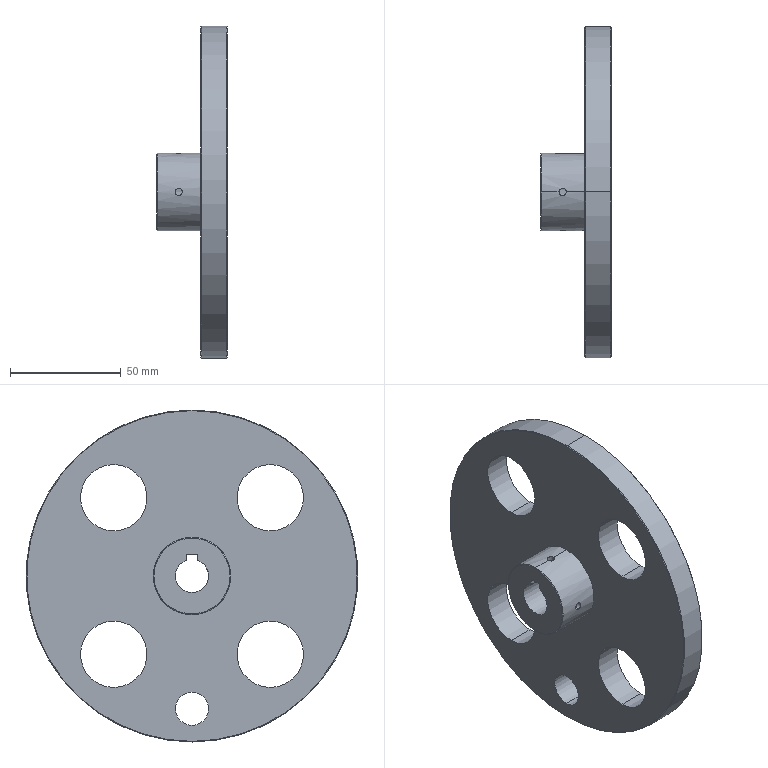Part | STEP file | 1 solid | 31 faces | box 32 x 150 x 150 mm | volume 189006 mm3 | cylinder 19 | cone 6 | plane 6 | commonest cylinder face diameters 30 x8 3.3 x4 15 x3 35 x2 150 x2